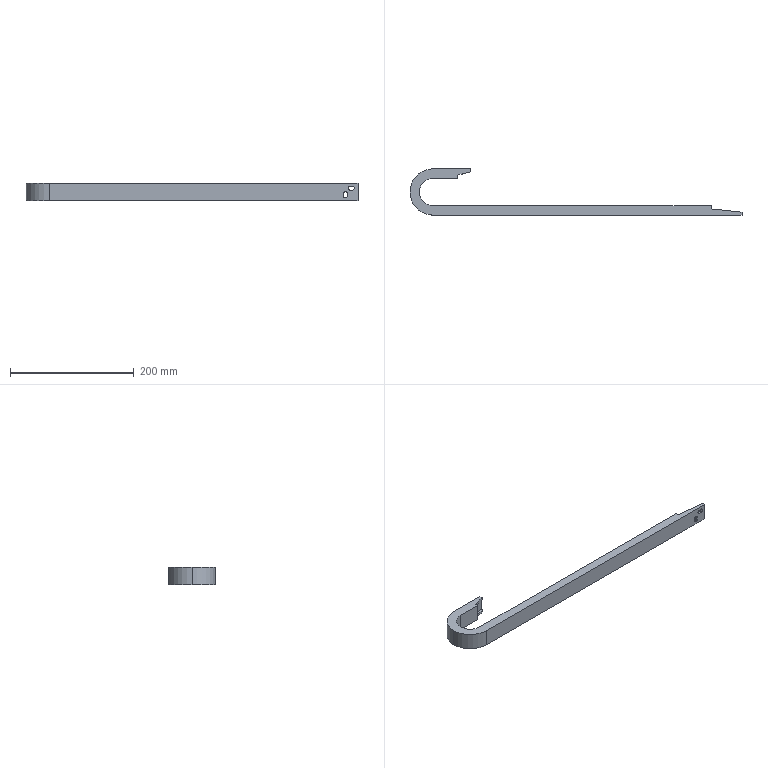Part | SolidWorks | features BaseBody 1 | 1 solid | 46 faces | box 537.6 x 75.2 x 28 mm | volume 139121 mm3 | plane 28 | cylinder 18 | commonest cylinder face diameters 6.5 x10 44.8 x2 50 x2 70 x2 75.2 x2
STEP:
#1=CARTESIAN_POINT('',(-460.45,65.,0.4));
#2=VERTEX_POINT('',#1);
#3=CARTESIAN_POINT('',(-457.2,65.,-2.85));
#4=VERTEX_POINT('',#3);
#5=CARTESIAN_POINT('',(-460.45,65.,-2.85));
#6=DIRECTION('',(0.,1.,0.));
#7=DIRECTION('',(0.,0.,-1.));
#8=AXIS2_PLACEMENT_3D('',#5,#6,#7);
#9=CIRCLE('',#8,3.25);
#10=EDGE_CURVE('',#2,#4,#9,.T.);
#11=ORIENTED_EDGE('',*,*,#10,.F.);
#12=CARTESIAN_POINT('',(-460.45,67.6,0.4));
#13=VERTEX_POINT('',#12);
#14=CARTESIAN_POINT('',(-460.45,-7.601,0.4));
#15=DIRECTION('',(0.,1.,0.));
#16=VECTOR('',#15,1000.);
#17=LINE('',#14,#16);
#18=EDGE_CURVE('',#2,#13,#17,.T.);
#19=ORIENTED_EDGE('',*,*,#18,.T.);
#20=CARTESIAN_POINT('',(-457.2,67.6,-2.85));
#21=VERTEX_POINT('',#20);
#22=CARTESIAN_POINT('',(-460.45,67.6,-2.85));
#23=DIRECTION('',(0.,1.,0.));
#24=DIRECTION('',(0.,0.,1.));
#25=AXIS2_PLACEMENT_3D('',#22,#23,#24);
#26=CIRCLE('',#25,3.25);
#27=EDGE_CURVE('',#13,#21,#26,.T.);
#28=ORIENTED_EDGE('',*,*,#27,.T.);
#29=CARTESIAN_POINT('',(-457.2,-7.601,-2.85));
#30=DIRECTION('',(0.,1.,0.));
#31=VECTOR('',#30,1000.);
#32=LINE('',#29,#31);
#33=EDGE_CURVE('',#4,#21,#32,.T.);
#34=ORIENTED_EDGE('',*,*,#33,.F.);
#35=EDGE_LOOP('',(#11,#19,#28,#34));
#36=FACE_OUTER_BOUND('',#35,.T.);
#37=CARTESIAN_POINT('',(-460.45,-7.601,-2.85));
#38=DIRECTION('',(0.,1.,0.));
#39=DIRECTION('',(0.,0.,1.));
#40=AXIS2_PLACEMENT_3D('',#37,#38,#39);
#41=CYLINDRICAL_SURFACE('',#40,3.25);
#42=ADVANCED_FACE('',(#36),#41,.F.);
#43=CARTESIAN_POINT('',(-20.45,-7.6,0.4));
#44=VERTEX_POINT('',#43);
#45=CARTESIAN_POINT('',(-17.2,-7.6,-2.85));
#46=VERTEX_POINT('',#45);
#47=CARTESIAN_POINT('',(-20.45,-7.6,-2.85));
#48=DIRECTION('',(0.,1.,0.));
#49=DIRECTION('',(0.,0.,1.));
#50=AXIS2_PLACEMENT_3D('',#47,#48,#49);
#51=CIRCLE('',#50,3.25);
#52=EDGE_CURVE('',#44,#46,#51,.T.);
#53=ORIENTED_EDGE('',*,*,#52,.F.);
#54=CARTESIAN_POINT('',(-20.45,-5.,0.4));
#55=VERTEX_POINT('',#54);
#56=CARTESIAN_POINT('',(-20.45,-7.6,0.4));
#57=DIRECTION('',(0.,1.,0.));
#58=VECTOR('',#57,1000.);
#59=LINE('',#56,#58);
#60=EDGE_CURVE('',#44,#55,#59,.T.);
#61=ORIENTED_EDGE('',*,*,#60,.T.);
#62=CARTESIAN_POINT('',(-17.2,-5.,-2.85));
#63=VERTEX_POINT('',#62);
#64=CARTESIAN_POINT('',(-20.45,-5.,-2.85));
#65=DIRECTION('',(0.,1.,0.));
#66=DIRECTION('',(0.,0.,1.));
#67=AXIS2_PLACEMENT_3D('',#64,#65,#66);
#68=CIRCLE('',#67,3.25);
#69=EDGE_CURVE('',#55,#63,#68,.T.);
#70=ORIENTED_EDGE('',*,*,#69,.T.);
#71=CARTESIAN_POINT('',(-17.2,-7.6,-2.85));
#72=DIRECTION('',(0.,1.,0.));
#73=VECTOR('',#72,1000.);
#74=LINE('',#71,#73);
#75=EDGE_CURVE('',#46,#63,#74,.T.);
#76=ORIENTED_EDGE('',*,*,#75,.F.);
#77=EDGE_LOOP('',(#53,#61,#70,#76));
#78=FACE_OUTER_BOUND('',#77,.T.);
#79=CARTESIAN_POINT('',(-20.45,-7.6,-2.85));
#80=DIRECTION('',(0.,1.,0.));
#81=DIRECTION('',(0.,0.,1.));
#82=AXIS2_PLACEMENT_3D('',#79,#80,#81);
#83=CYLINDRICAL_SURFACE('',#82,3.25);
#84=ADVANCED_FACE('',(#78),#83,.F.);
#85=CARTESIAN_POINT('',(-500.,-7.6,14.));
#86=VERTEX_POINT('',#85);
#87=CARTESIAN_POINT('',(-537.6,30.,14.));
#88=VERTEX_POINT('',#87);
#89=CARTESIAN_POINT('',(-500.,30.,14.));
#90=DIRECTION('',(0.,0.,-1.));
#91=DIRECTION('',(-1.,0.,0.));
#92=AXIS2_PLACEMENT_3D('',#89,#90,#91);
#93=CIRCLE('',#92,37.6);
#94=EDGE_CURVE('',#86,#88,#93,.T.);
#95=ORIENTED_EDGE('',*,*,#94,.T.);
#96=CARTESIAN_POINT('',(-537.6,30.,-14.));
#97=VERTEX_POINT('',#96);
#98=CARTESIAN_POINT('',(-537.6,30.,0.));
#99=DIRECTION('',(0.,0.,-1.));
#100=VECTOR('',#99,1000.);
#101=LINE('',#98,#100);
#102=EDGE_CURVE('',#88,#97,#101,.T.);
#103=ORIENTED_EDGE('',*,*,#102,.T.);
#104=CARTESIAN_POINT('',(-500.,-7.6,-14.));
#105=VERTEX_POINT('',#104);
#106=CARTESIAN_POINT('',(-500.,30.,-14.));
#107=DIRECTION('',(0.,0.,-1.));
#108=DIRECTION('',(-1.,0.,0.));
#109=AXIS2_PLACEMENT_3D('',#106,#107,#108);
#110=CIRCLE('',#109,37.6);
#111=EDGE_CURVE('',#105,#97,#110,.T.);
#112=ORIENTED_EDGE('',*,*,#111,.F.);
#113=CARTESIAN_POINT('',(-500.,-7.6,-14.));
#114=DIRECTION('',(0.,0.,-1.));
#115=VECTOR('',#114,1000.);
#116=LINE('',#113,#115);
#117=EDGE_CURVE('',#86,#105,#116,.T.);
#118=ORIENTED_EDGE('',*,*,#117,.F.);
#119=EDGE_LOOP('',(#95,#103,#112,#118));
#120=FACE_OUTER_BOUND('',#119,.T.);
#121=CARTESIAN_POINT('',(-500.,30.,0.));
#122=DIRECTION('',(0.,0.,-1.));
#123=DIRECTION('',(-1.,0.,0.));
#124=AXIS2_PLACEMENT_3D('',#121,#122,#123);
#125=CYLINDRICAL_SURFACE('',#124,37.6);
#126=ADVANCED_FACE('',(#120),#125,.T.);
#127=CARTESIAN_POINT('',(-522.4,30.,14.));
#128=VERTEX_POINT('',#127);
#129=CARTESIAN_POINT('',(-500.,52.4,14.));
#130=VERTEX_POINT('',#129);
#131=CARTESIAN_POINT('',(-500.,30.,14.));
#132=DIRECTION('',(0.,0.,-1.));
#133=DIRECTION('',(-1.,0.,0.));
#134=AXIS2_PLACEMENT_3D('',#131,#132,#133);
#135=CIRCLE('',#134,22.4);
#136=EDGE_CURVE('',#128,#130,#135,.T.);
#137=ORIENTED_EDGE('',*,*,#136,.F.);
#138=CARTESIAN_POINT('',(-522.4,30.,-14.));
#139=VERTEX_POINT('',#138);
#140=CARTESIAN_POINT('',(-522.4,30.,0.));
#141=DIRECTION('',(0.,0.,-1.));
#142=VECTOR('',#141,1000.);
#143=LINE('',#140,#142);
#144=EDGE_CURVE('',#128,#139,#143,.T.);
#145=ORIENTED_EDGE('',*,*,#144,.T.);
#146=CARTESIAN_POINT('',(-500.,52.4,-14.));
#147=VERTEX_POINT('',#146);
#148=CARTESIAN_POINT('',(-500.,30.,-14.));
#149=DIRECTION('',(0.,0.,-1.));
#150=DIRECTION('',(-1.,0.,0.));
#151=AXIS2_PLACEMENT_3D('',#148,#149,#150);
#152=CIRCLE('',#151,22.4);
#153=EDGE_CURVE('',#139,#147,#152,.T.);
#154=ORIENTED_EDGE('',*,*,#153,.T.);
#155=CARTESIAN_POINT('',(-500.,52.4,-14.));
#156=DIRECTION('',(0.,0.,1.));
#157=VECTOR('',#156,1000.);
#158=LINE('',#155,#157);
#159=EDGE_CURVE('',#147,#130,#158,.T.);
#160=ORIENTED_EDGE('',*,*,#159,.T.);
#161=EDGE_LOOP('',(#137,#145,#154,#160));
#162=FACE_OUTER_BOUND('',#161,.T.);
#163=CARTESIAN_POINT('',(-500.,30.,0.));
#164=DIRECTION('',(0.,0.,-1.));
#165=DIRECTION('',(-1.,0.,0.));
#166=AXIS2_PLACEMENT_3D('',#163,#164,#165);
#167=CYLINDRICAL_SURFACE('',#166,22.4);
#168=ADVANCED_FACE('',(#162),#167,.F.);
#169=CARTESIAN_POINT('',(-500.,5.,10.));
#170=VERTEX_POINT('',#169);
#171=CARTESIAN_POINT('',(-525.,30.,10.));
#172=VERTEX_POINT('',#171);
#173=CARTESIAN_POINT('',(-500.,30.,10.));
#174=DIRECTION('',(0.,0.,-1.));
#175=DIRECTION('',(-1.,0.,0.));
#176=AXIS2_PLACEMENT_3D('',#173,#174,#175);
#177=CIRCLE('',#176,25.);
#178=EDGE_CURVE('',#170,#172,#177,.T.);
#179=ORIENTED_EDGE('',*,*,#178,.T.);
#180=CARTESIAN_POINT('',(-525.,30.,-10.));
#181=VERTEX_POINT('',#180);
#182=CARTESIAN_POINT('',(-525.,30.,0.));
#183=DIRECTION('',(0.,0.,-1.));
#184=VECTOR('',#183,1000.);
#185=LINE('',#182,#184);
#186=EDGE_CURVE('',#172,#181,#185,.T.);
#187=ORIENTED_EDGE('',*,*,#186,.T.);
#188=CARTESIAN_POINT('',(-500.,5.,-10.));
#189=VERTEX_POINT('',#188);
#190=CARTESIAN_POINT('',(-500.,30.,-10.));
#191=DIRECTION('',(0.,0.,-1.));
#192=DIRECTION('',(-1.,0.,0.));
#193=AXIS2_PLACEMENT_3D('',#190,#191,#192);
#194=CIRCLE('',#193,25.);
#195=EDGE_CURVE('',#189,#181,#194,.T.);
#196=ORIENTED_EDGE('',*,*,#195,.F.);
#197=CARTESIAN_POINT('',(-500.,5.,-10.));
#198=DIRECTION('',(0.,0.,1.));
#199=VECTOR('',#198,1000.);
#200=LINE('',#197,#199);
#201=EDGE_CURVE('',#189,#170,#200,.T.);
#202=ORIENTED_EDGE('',*,*,#201,.T.);
#203=EDGE_LOOP('',(#179,#187,#196,#202));
#204=FACE_OUTER_BOUND('',#203,.T.);
#205=CARTESIAN_POINT('',(-500.,30.,0.));
#206=DIRECTION('',(0.,0.,-1.));
#207=DIRECTION('',(-1.,0.,0.));
#208=AXIS2_PLACEMENT_3D('',#205,#206,#207);
#209=CYLINDRICAL_SURFACE('',#208,25.);
#210=ADVANCED_FACE('',(#204),#209,.T.);
#211=CARTESIAN_POINT('',(-535.,30.,10.));
#212=VERTEX_POINT('',#211);
#213=CARTESIAN_POINT('',(-500.,65.,10.));
#214=VERTEX_POINT('',#213);
#215=CARTESIAN_POINT('',(-500.,30.,10.));
#216=DIRECTION('',(0.,0.,-1.));
#217=DIRECTION('',(-1.,0.,0.));
#218=AXIS2_PLACEMENT_3D('',#215,#216,#217);
#219=CIRCLE('',#218,35.);
#220=EDGE_CURVE('',#212,#214,#219,.T.);
#221=ORIENTED_EDGE('',*,*,#220,.F.);
#222=CARTESIAN_POINT('',(-535.,30.,-10.));
#223=VERTEX_POINT('',#222);
#224=CARTESIAN_POINT('',(-535.,30.,0.));
#225=DIRECTION('',(0.,0.,-1.));
#226=VECTOR('',#225,1000.);
#227=LINE('',#224,#226);
#228=EDGE_CURVE('',#212,#223,#227,.T.);
#229=ORIENTED_EDGE('',*,*,#228,.T.);
#230=CARTESIAN_POINT('',(-500.,65.,-10.));
#231=VERTEX_POINT('',#230);
#232=CARTESIAN_POINT('',(-500.,30.,-10.));
#233=DIRECTION('',(0.,0.,-1.));
#234=DIRECTION('',(-1.,0.,0.));
#235=AXIS2_PLACEMENT_3D('',#232,#233,#234);
#236=CIRCLE('',#235,35.);
#237=EDGE_CURVE('',#223,#231,#236,.T.);
#238=ORIENTED_EDGE('',*,*,#237,.T.);
#239=CARTESIAN_POINT('',(-500.,65.,-10.));
#240=DIRECTION('',(0.,0.,-1.));
#241=VECTOR('',#240,1000.);
#242=LINE('',#239,#241);
#243=EDGE_CURVE('',#214,#231,#242,.T.);
#244=ORIENTED_EDGE('',*,*,#243,.F.);
#245=EDGE_LOOP('',(#221,#229,#238,#244));
#246=FACE_OUTER_BOUND('',#245,.T.);
#247=CARTESIAN_POINT('',(-500.,30.,0.));
#248=DIRECTION('',(0.,0.,-1.));
#249=DIRECTION('',(-1.,0.,0.));
#250=AXIS2_PLACEMENT_3D('',#247,#248,#249);
#251=CYLINDRICAL_SURFACE('',#250,35.);
#252=ADVANCED_FACE('',(#246),#251,.F.);
#253=CARTESIAN_POINT('',(-452.75,65.,3.1));
#254=VERTEX_POINT('',#253);
#255=CARTESIAN_POINT('',(-452.75,65.,9.6));
#256=VERTEX_POINT('',#255);
#257=CARTESIAN_POINT('',(-452.75,65.,6.35));
#258=DIRECTION('',(0.,1.,0.));
#259=DIRECTION('',(0.,0.,-1.));
#260=AXIS2_PLACEMENT_3D('',#257,#258,#259);
#261=CIRCLE('',#260,3.25);
#262=EDGE_CURVE('',#254,#256,#261,.T.);
#263=ORIENTED_EDGE('',*,*,#262,.T.);
#264=CARTESIAN_POINT('',(-449.25,65.,9.6));
#265=VERTEX_POINT('',#264);
#266=CARTESIAN_POINT('',(-452.75,65.,9.6));
#267=DIRECTION('',(1.,0.,0.));
#268=VECTOR('',#267,1000.);
#269=LINE('',#266,#268);
#270=EDGE_CURVE('',#256,#265,#269,.T.);
#271=ORIENTED_EDGE('',*,*,#270,.T.);
#272=CARTESIAN_POINT('',(-449.25,65.,3.1));
#273=VERTEX_POINT('',#272);
#274=CARTESIAN_POINT('',(-449.25,65.,6.35));
#275=DIRECTION('',(0.,1.,0.));
#276=DIRECTION('',(0.,0.,-1.));
#277=AXIS2_PLACEMENT_3D('',#274,#275,#276);
#278=CIRCLE('',#277,3.25);
#279=EDGE_CURVE('',#265,#273,#278,.T.);
#280=ORIENTED_EDGE('',*,*,#279,.T.);
#281=CARTESIAN_POINT('',(-452.75,65.,3.1));
#282=DIRECTION('',(-1.,0.,0.));
#283=VECTOR('',#282,1000.);
#284=LINE('',#281,#283);
#285=EDGE_CURVE('',#273,#254,#284,.T.);
#286=ORIENTED_EDGE('',*,*,#285,.T.);
#287=EDGE_LOOP('',(#263,#271,#280,#286));
#288=FACE_BOUND('',#287,.T.);
#289=CARTESIAN_POINT('',(-457.2,65.,-6.35));
#290=VERTEX_POINT('',#289);
#291=CARTESIAN_POINT('',(-463.7,65.,-6.35));
#292=VERTEX_POINT('',#291);
#293=CARTESIAN_POINT('',(-460.45,65.,-6.35));
#294=DIRECTION('',(0.,1.,0.));
#295=DIRECTION('',(0.,0.,-1.));
#296=AXIS2_PLACEMENT_3D('',#293,#294,#295);
#297=CIRCLE('',#296,3.25);
#298=EDGE_CURVE('',#290,#292,#297,.T.);
#299=ORIENTED_EDGE('',*,*,#298,.T.);
#300=CARTESIAN_POINT('',(-463.7,65.,-2.85));
#301=VERTEX_POINT('',#300);
#302=CARTESIAN_POINT('',(-463.7,65.,-6.35));
#303=DIRECTION('',(0.,0.,1.));
#304=VECTOR('',#303,1000.);
#305=LINE('',#302,#304);
#306=EDGE_CURVE('',#292,#301,#305,.T.);
#307=ORIENTED_EDGE('',*,*,#306,.T.);
#308=CARTESIAN_POINT('',(-460.45,65.,-2.85));
#309=DIRECTION('',(0.,1.,0.));
#310=DIRECTION('',(0.,0.,-1.));
#311=AXIS2_PLACEMENT_3D('',#308,#309,#310);
#312=CIRCLE('',#311,3.25);
#313=EDGE_CURVE('',#301,#2,#312,.T.);
#314=ORIENTED_EDGE('',*,*,#313,.T.);
#315=ORIENTED_EDGE('',*,*,#10,.T.);
#316=CARTESIAN_POINT('',(-457.2,65.,-6.35));
#317=DIRECTION('',(0.,0.,-1.));
#318=VECTOR('',#317,1000.);
#319=LINE('',#316,#318);
#320=EDGE_CURVE('',#4,#290,#319,.T.);
#321=ORIENTED_EDGE('',*,*,#320,.T.);
#322=EDGE_LOOP('',(#299,#307,#314,#315,#321));
#323=FACE_BOUND('',#322,.T.);
#324=ORIENTED_EDGE('',*,*,#243,.T.);
#325=CARTESIAN_POINT('',(-440.,65.,-10.));
#326=VERTEX_POINT('',#325);
#327=CARTESIAN_POINT('',(-500.,65.,-10.));
#328=DIRECTION('',(1.,0.,0.));
#329=VECTOR('',#328,1000.);
#330=LINE('',#327,#329);
#331=EDGE_CURVE('',#231,#326,#330,.T.);
#332=ORIENTED_EDGE('',*,*,#331,.T.);
#333=CARTESIAN_POINT('',(-440.,65.,10.));
#334=VERTEX_POINT('',#333);
#335=CARTESIAN_POINT('',(-440.,65.,-10.));
#336=DIRECTION('',(0.,0.,-1.));
#337=VECTOR('',#336,1000.);
#338=LINE('',#335,#337);
#339=EDGE_CURVE('',#334,#326,#338,.T.);
#340=ORIENTED_EDGE('',*,*,#339,.F.);
#341=CARTESIAN_POINT('',(-500.,65.,10.));
#342=DIRECTION('',(1.,0.,0.));
#343=VECTOR('',#342,1000.);
#344=LINE('',#341,#343);
#345=EDGE_CURVE('',#214,#334,#344,.T.);
#346=ORIENTED_EDGE('',*,*,#345,.F.);
#347=EDGE_LOOP('',(#324,#332,#340,#346));
#348=FACE_OUTER_BOUND('',#347,.T.);
#349=CARTESIAN_POINT('',(-500.,65.,-10.));
#350=DIRECTION('',(0.,-1.,0.));
#351=DIRECTION('',(0.,0.,-1.));
#352=AXIS2_PLACEMENT_3D('',#349,#350,#351);
#353=PLANE('',#352);
#354=ADVANCED_FACE('',(#288,#323,#348),#353,.T.);
#355=CARTESIAN_POINT('',(-460.,55.,-10.));
#356=VERTEX_POINT('',#355);
#357=CARTESIAN_POINT('',(-460.,55.,10.));
#358=VERTEX_POINT('',#357);
#359=CARTESIAN_POINT('',(-460.,55.,-10.));
#360=DIRECTION('',(0.,0.,1.));
#361=VECTOR('',#360,1000.);
#362=LINE('',#359,#361);
#363=EDGE_CURVE('',#356,#358,#362,.T.);
#364=ORIENTED_EDGE('',*,*,#363,.F.);
#365=CARTESIAN_POINT('',(-500.,55.,-10.));
#366=VERTEX_POINT('',#365);
#367=CARTESIAN_POINT('',(-500.,55.,-10.));
#368=DIRECTION('',(1.,0.,0.));
#369=VECTOR('',#368,1000.);
#370=LINE('',#367,#369);
#371=EDGE_CURVE('',#366,#356,#370,.T.);
#372=ORIENTED_EDGE('',*,*,#371,.F.);
#373=CARTESIAN_POINT('',(-500.,55.,10.));
#374=VERTEX_POINT('',#373);
#375=CARTESIAN_POINT('',(-500.,55.,-10.));
#376=DIRECTION('',(0.,0.,1.));
#377=VECTOR('',#376,1000.);
#378=LINE('',#375,#377);
#379=EDGE_CURVE('',#366,#374,#378,.T.);
#380=ORIENTED_EDGE('',*,*,#379,.T.);
#381=CARTESIAN_POINT('',(-500.,55.,10.));
#382=DIRECTION('',(1.,0.,0.));
#383=VECTOR('',#382,1000.);
#384=LINE('',#381,#383);
#385=EDGE_CURVE('',#374,#358,#384,.T.);
#386=ORIENTED_EDGE('',*,*,#385,.T.);
#387=EDGE_LOOP('',(#364,#372,#380,#386));
#388=FACE_OUTER_BOUND('',#387,.T.);
#389=CARTESIAN_POINT('',(-500.,55.,-10.));
#390=DIRECTION('',(0.,1.,0.));
#391=DIRECTION('',(0.,0.,1.));
#392=AXIS2_PLACEMENT_3D('',#389,#390,#391);
#393=PLANE('',#392);
#394=ADVANCED_FACE('',(#388),#393,.T.);
#395=CARTESIAN_POINT('',(-460.,52.4,-14.));
#396=VERTEX_POINT('',#395);
#397=CARTESIAN_POINT('',(-500.,52.4,-14.));
#398=DIRECTION('',(1.,0.,0.));
#399=VECTOR('',#398,1000.);
#400=LINE('',#397,#399);
#401=EDGE_CURVE('',#147,#396,#400,.T.);
#402=ORIENTED_EDGE('',*,*,#401,.T.);
#403=CARTESIAN_POINT('',(-460.,52.4,14.));
#404=VERTEX_POINT('',#403);
#405=CARTESIAN_POINT('',(-460.,52.4,-14.));
#406=DIRECTION('',(0.,0.,1.));
#407=VECTOR('',#406,1000.);
#408=LINE('',#405,#407);
#409=EDGE_CURVE('',#396,#404,#408,.T.);
#410=ORIENTED_EDGE('',*,*,#409,.T.);
#411=CARTESIAN_POINT('',(-500.,52.4,14.));
#412=DIRECTION('',(1.,0.,0.));
#413=VECTOR('',#412,1000.);
#414=LINE('',#411,#413);
#415=EDGE_CURVE('',#130,#404,#414,.T.);
#416=ORIENTED_EDGE('',*,*,#415,.F.);
#417=ORIENTED_EDGE('',*,*,#159,.F.);
#418=EDGE_LOOP('',(#402,#410,#416,#417));
#419=FACE_OUTER_BOUND('',#418,.T.);
#420=CARTESIAN_POINT('',(-500.,52.4,-14.));
#421=DIRECTION('',(0.,1.,0.));
#422=DIRECTION('',(0.,0.,1.));
#423=AXIS2_PLACEMENT_3D('',#420,#421,#422);
#424=PLANE('',#423);
#425=ADVANCED_FACE('',(#419),#424,.F.);
#426=CARTESIAN_POINT('',(-452.75,67.6,9.6));
#427=VERTEX_POINT('',#426);
#428=CARTESIAN_POINT('',(-449.25,67.6,9.6));
#429=VERTEX_POINT('',#428);
#430=CARTESIAN_POINT('',(-452.75,67.6,9.6));
#431=DIRECTION('',(1.,0.,0.));
#432=VECTOR('',#431,1000.);
#433=LINE('',#430,#432);
#434=EDGE_CURVE('',#427,#429,#433,.T.);
#435=ORIENTED_EDGE('',*,*,#434,.F.);
#436=CARTESIAN_POINT('',(-452.75,67.6,3.1));
#437=VERTEX_POINT('',#436);
#438=CARTESIAN_POINT('',(-452.75,67.6,6.35));
#439=DIRECTION('',(0.,1.,0.));
#440=DIRECTION('',(0.,0.,1.));
#441=AXIS2_PLACEMENT_3D('',#438,#439,#440);
#442=CIRCLE('',#441,3.25);
#443=EDGE_CURVE('',#437,#427,#442,.T.);
#444=ORIENTED_EDGE('',*,*,#443,.F.);
#445=CARTESIAN_POINT('',(-449.25,67.6,3.1));
#446=VERTEX_POINT('',#445);
#447=CARTESIAN_POINT('',(-452.75,67.6,3.1));
#448=DIRECTION('',(-1.,0.,0.));
#449=VECTOR('',#448,1000.);
#450=LINE('',#447,#449);
#451=EDGE_CURVE('',#446,#437,#450,.T.);
#452=ORIENTED_EDGE('',*,*,#451,.F.);
#453=CARTESIAN_POINT('',(-449.25,67.6,6.35));
#454=DIRECTION('',(0.,1.,0.));
#455=DIRECTION('',(0.,0.,1.));
#456=AXIS2_PLACEMENT_3D('',#453,#454,#455);
#457=CIRCLE('',#456,3.25);
#458=EDGE_CURVE('',#429,#446,#457,.T.);
#459=ORIENTED_EDGE('',*,*,#458,.F.);
#460=EDGE_LOOP('',(#435,#444,#452,#459));
#461=FACE_BOUND('',#460,.T.);
#462=CARTESIAN_POINT('',(-463.7,67.6,-6.35));
#463=VERTEX_POINT('',#462);
#464=CARTESIAN_POINT('',(-463.7,67.6,-2.85));
#465=VERTEX_POINT('',#464);
#466=CARTESIAN_POINT('',(-463.7,67.6,-6.35));
#467=DIRECTION('',(0.,0.,1.));
#468=VECTOR('',#467,1000.);
#469=LINE('',#466,#468);
#470=EDGE_CURVE('',#463,#465,#469,.T.);
#471=ORIENTED_EDGE('',*,*,#470,.F.);
#472=CARTESIAN_POINT('',(-457.2,67.6,-6.35));
#473=VERTEX_POINT('',#472);
#474=CARTESIAN_POINT('',(-460.45,67.6,-6.35));
#475=DIRECTION('',(0.,1.,0.));
#476=DIRECTION('',(0.,0.,1.));
#477=AXIS2_PLACEMENT_3D('',#474,#475,#476);
#478=CIRCLE('',#477,3.25);
#479=EDGE_CURVE('',#473,#463,#478,.T.);
#480=ORIENTED_EDGE('',*,*,#479,.F.);
#481=CARTESIAN_POINT('',(-457.2,67.6,-6.35));
#482=DIRECTION('',(0.,0.,-1.));
#483=VECTOR('',#482,1000.);
#484=LINE('',#481,#483);
#485=EDGE_CURVE('',#21,#473,#484,.T.);
#486=ORIENTED_EDGE('',*,*,#485,.F.);
#487=ORIENTED_EDGE('',*,*,#27,.F.);
#488=CARTESIAN_POINT('',(-460.45,67.6,-2.85));
#489=DIRECTION('',(0.,1.,0.));
#490=DIRECTION('',(0.,0.,1.));
#491=AXIS2_PLACEMENT_3D('',#488,#489,#490);
#492=CIRCLE('',#491,3.25);
#493=EDGE_CURVE('',#465,#13,#492,.T.);
#494=ORIENTED_EDGE('',*,*,#493,.F.);
#495=EDGE_LOOP('',(#471,#480,#486,#487,#494));
#496=FACE_BOUND('',#495,.T.);
#497=CARTESIAN_POINT('',(-500.,67.6,14.));
#498=VERTEX_POINT('',#497);
#499=CARTESIAN_POINT('',(-500.,67.6,-14.));
#500=VERTEX_POINT('',#499);
#501=CARTESIAN_POINT('',(-500.,67.6,-14.));
#502=DIRECTION('',(0.,0.,-1.));
#503=VECTOR('',#502,1000.);
#504=LINE('',#501,#503);
#505=EDGE_CURVE('',#498,#500,#504,.T.);
#506=ORIENTED_EDGE('',*,*,#505,.F.);
#507=CARTESIAN_POINT('',(-440.,67.6,14.));
#508=VERTEX_POINT('',#507);
#509=CARTESIAN_POINT('',(-500.,67.6,14.));
#510=DIRECTION('',(1.,0.,0.));
#511=VECTOR('',#510,1000.);
#512=LINE('',#509,#511);
#513=EDGE_CURVE('',#498,#508,#512,.T.);
#514=ORIENTED_EDGE('',*,*,#513,.T.);
#515=CARTESIAN_POINT('',(-440.,67.6,-14.));
#516=VERTEX_POINT('',#515);
#517=CARTESIAN_POINT('',(-440.,67.6,-14.));
#518=DIRECTION('',(0.,0.,-1.));
#519=VECTOR('',#518,1000.);
#520=LINE('',#517,#519);
#521=EDGE_CURVE('',#508,#516,#520,.T.);
#522=ORIENTED_EDGE('',*,*,#521,.T.);
#523=CARTESIAN_POINT('',(-500.,67.6,-14.));
#524=DIRECTION('',(1.,0.,0.));
#525=VECTOR('',#524,1000.);
#526=LINE('',#523,#525);
#527=EDGE_CURVE('',#500,#516,#526,.T.);
#528=ORIENTED_EDGE('',*,*,#527,.F.);
#529=EDGE_LOOP('',(#506,#514,#522,#528));
#530=FACE_OUTER_BOUND('',#529,.T.);
#531=CARTESIAN_POINT('',(-500.,67.6,-14.));
#532=DIRECTION('',(0.,-1.,0.));
#533=DIRECTION('',(0.,0.,-1.));
#534=AXIS2_PLACEMENT_3D('',#531,#532,#533);
#535=PLANE('',#534);
#536=ADVANCED_FACE('',(#461,#496,#530),#535,.F.);
#537=ORIENTED_EDGE('',*,*,#228,.F.);
#538=CARTESIAN_POINT('',(-500.,-5.,10.));
#539=VERTEX_POINT('',#538);
#540=CARTESIAN_POINT('',(-500.,30.,10.));
#541=DIRECTION('',(0.,0.,-1.));
#542=DIRECTION('',(-1.,0.,0.));
#543=AXIS2_PLACEMENT_3D('',#540,#541,#542);
#544=CIRCLE('',#543,35.);
#545=EDGE_CURVE('',#539,#212,#544,.T.);
#546=ORIENTED_EDGE('',*,*,#545,.F.);
#547=CARTESIAN_POINT('',(-500.,-5.,-10.));
#548=VERTEX_POINT('',#547);
#549=CARTESIAN_POINT('',(-500.,-5.,-10.));
#550=DIRECTION('',(0.,0.,-1.));
#551=VECTOR('',#550,1000.);
#552=LINE('',#549,#551);
#553=EDGE_CURVE('',#539,#548,#552,.T.);
#554=ORIENTED_EDGE('',*,*,#553,.T.);
#555=CARTESIAN_POINT('',(-500.,30.,-10.));
#556=DIRECTION('',(0.,0.,-1.));
#557=DIRECTION('',(-1.,0.,0.));
#558=AXIS2_PLACEMENT_3D('',#555,#556,#557);
#559=CIRCLE('',#558,35.);
#560=EDGE_CURVE('',#548,#223,#559,.T.);
#561=ORIENTED_EDGE('',*,*,#560,.T.);
#562=EDGE_LOOP('',(#537,#546,#554,#561));
#563=FACE_OUTER_BOUND('',#562,.T.);
#564=CARTESIAN_POINT('',(-500.,30.,0.));
#565=DIRECTION('',(0.,0.,-1.));
#566=DIRECTION('',(-1.,0.,0.));
#567=AXIS2_PLACEMENT_3D('',#564,#565,#566);
#568=CYLINDRICAL_SURFACE('',#567,35.);
#569=ADVANCED_FACE('',(#563),#568,.F.);
#570=ORIENTED_EDGE('',*,*,#186,.F.);
#571=CARTESIAN_POINT('',(-500.,30.,10.));
#572=DIRECTION('',(0.,0.,-1.));
#573=DIRECTION('',(-1.,0.,0.));
#574=AXIS2_PLACEMENT_3D('',#571,#572,#573);
#575=CIRCLE('',#574,25.);
#576=EDGE_CURVE('',#172,#374,#575,.T.);
#577=ORIENTED_EDGE('',*,*,#576,.T.);
#578=ORIENTED_EDGE('',*,*,#379,.F.);
#579=CARTESIAN_POINT('',(-500.,30.,-10.));
#580=DIRECTION('',(0.,0.,-1.));
#581=DIRECTION('',(-1.,0.,0.));
#582=AXIS2_PLACEMENT_3D('',#579,#580,#581);
#583=CIRCLE('',#582,25.);
#584=EDGE_CURVE('',#181,#366,#583,.T.);
#585=ORIENTED_EDGE('',*,*,#584,.F.);
#586=EDGE_LOOP('',(#570,#577,#578,#585));
#587=FACE_OUTER_BOUND('',#586,.T.);
#588=CARTESIAN_POINT('',(-500.,30.,0.));
#589=DIRECTION('',(0.,0.,-1.));
#590=DIRECTION('',(-1.,0.,0.));
#591=AXIS2_PLACEMENT_3D('',#588,#589,#590);
#592=CYLINDRICAL_SURFACE('',#591,25.);
#593=ADVANCED_FACE('',(#587),#592,.T.);
#594=ORIENTED_EDGE('',*,*,#144,.F.);
#595=CARTESIAN_POINT('',(-500.,7.6,14.));
#596=VERTEX_POINT('',#595);
#597=CARTESIAN_POINT('',(-500.,30.,14.));
#598=DIRECTION('',(0.,0.,-1.));
#599=DIRECTION('',(-1.,0.,0.));
#600=AXIS2_PLACEMENT_3D('',#597,#598,#599);
#601=CIRCLE('',#600,22.4);
#602=EDGE_CURVE('',#596,#128,#601,.T.);
#603=ORIENTED_EDGE('',*,*,#602,.F.);
#604=CARTESIAN_POINT('',(-500.,7.6,-14.));
#605=VERTEX_POINT('',#604);
#606=CARTESIAN_POINT('',(-500.,7.6,-14.));
#607=DIRECTION('',(0.,0.,1.));
#608=VECTOR('',#607,1000.);
#609=LINE('',#606,#608);
#610=EDGE_CURVE('',#605,#596,#609,.T.);
#611=ORIENTED_EDGE('',*,*,#610,.F.);
#612=CARTESIAN_POINT('',(-500.,30.,-14.));
#613=DIRECTION('',(0.,0.,-1.));
#614=DIRECTION('',(-1.,0.,0.));
#615=AXIS2_PLACEMENT_3D('',#612,#613,#614);
#616=CIRCLE('',#615,22.4);
#617=EDGE_CURVE('',#605,#139,#616,.T.);
#618=ORIENTED_EDGE('',*,*,#617,.T.);
#619=EDGE_LOOP('',(#594,#603,#611,#618));
#620=FACE_OUTER_BOUND('',#619,.T.);
#621=CARTESIAN_POINT('',(-500.,30.,0.));
#622=DIRECTION('',(0.,0.,-1.));
#623=DIRECTION('',(-1.,0.,0.));
#624=AXIS2_PLACEMENT_3D('',#621,#622,#623);
#625=CYLINDRICAL_SURFACE('',#624,22.4);
#626=ADVANCED_FACE('',(#620),#625,.F.);
#627=ORIENTED_EDGE('',*,*,#102,.F.);
#628=CARTESIAN_POINT('',(-500.,30.,14.));
#629=DIRECTION('',(0.,0.,-1.));
#630=DIRECTION('',(-1.,0.,0.));
#631=AXIS2_PLACEMENT_3D('',#628,#629,#630);
#632=CIRCLE('',#631,37.6);
#633=EDGE_CURVE('',#88,#498,#632,.T.);
#634=ORIENTED_EDGE('',*,*,#633,.T.);
#635=ORIENTED_EDGE('',*,*,#505,.T.);
#636=CARTESIAN_POINT('',(-500.,30.,-14.));
#637=DIRECTION('',(0.,0.,-1.));
#638=DIRECTION('',(-1.,0.,0.));
#639=AXIS2_PLACEMENT_3D('',#636,#637,#638);
#640=CIRCLE('',#639,37.6);
#641=EDGE_CURVE('',#97,#500,#640,.T.);
#642=ORIENTED_EDGE('',*,*,#641,.F.);
#643=EDGE_LOOP('',(#627,#634,#635,#642));
#644=FACE_OUTER_BOUND('',#643,.T.);
#645=CARTESIAN_POINT('',(-500.,30.,0.));
#646=DIRECTION('',(0.,0.,-1.));
#647=DIRECTION('',(-1.,0.,0.));
#648=AXIS2_PLACEMENT_3D('',#645,#646,#647);
#649=CYLINDRICAL_SURFACE('',#648,37.6);
#650=ADVANCED_FACE('',(#644),#649,.T.);
#651=CARTESIAN_POINT('',(-50.,5.,10.));
#652=VERTEX_POINT('',#651);
#653=CARTESIAN_POINT('',(-50.,2.6,10.));
#654=VERTEX_POINT('',#653);
#655=CARTESIAN_POINT('',(-50.,5.,10.));
#656=DIRECTION('',(0.,-1.,0.));
#657=VECTOR('',#656,1000.);
#658=LINE('',#655,#657);
#659=EDGE_CURVE('',#652,#654,#658,.T.);
#660=ORIENTED_EDGE('',*,*,#659,.T.);
#661=CARTESIAN_POINT('',(0.,-2.6,10.));
#662=VERTEX_POINT('',#661);
#663=CARTESIAN_POINT('',(-495.432,48.925,10.));
#664=DIRECTION('',(0.9946,-0.1034,0.));
#665=VECTOR('',#664,1000.);
#666=LINE('',#663,#665);
#667=EDGE_CURVE('',#654,#662,#666,.T.);
#668=ORIENTED_EDGE('',*,*,#667,.T.);
#669=CARTESIAN_POINT('',(0.,-5.,10.));
#670=VERTEX_POINT('',#669);
#671=CARTESIAN_POINT('',(0.,5.,10.));
#672=DIRECTION('',(0.,-1.,0.));
#673=VECTOR('',#672,1000.);
#674=LINE('',#671,#673);
#675=EDGE_CURVE('',#662,#670,#674,.T.);
#676=ORIENTED_EDGE('',*,*,#675,.T.);
#677=CARTESIAN_POINT('',(-500.,-5.,10.));
#678=DIRECTION('',(1.,0.,0.));
#679=VECTOR('',#678,1000.);
#680=LINE('',#677,#679);
#681=EDGE_CURVE('',#539,#670,#680,.T.);
#682=ORIENTED_EDGE('',*,*,#681,.F.);
#683=ORIENTED_EDGE('',*,*,#545,.T.);
#684=ORIENTED_EDGE('',*,*,#220,.T.);
#685=ORIENTED_EDGE('',*,*,#345,.T.);
#686=CARTESIAN_POINT('',(-440.,62.6,10.));
#687=VERTEX_POINT('',#686);
#688=CARTESIAN_POINT('',(-440.,55.,10.));
#689=DIRECTION('',(0.,1.,0.));
#690=VECTOR('',#689,1000.);
#691=LINE('',#688,#690);
#692=EDGE_CURVE('',#687,#334,#691,.T.);
#693=ORIENTED_EDGE('',*,*,#692,.F.);
#694=CARTESIAN_POINT('',(-460.,57.4,10.));
#695=VERTEX_POINT('',#694);
#696=CARTESIAN_POINT('',(-510.229,44.341,10.));
#697=DIRECTION('',(-0.9678,-0.2516,0.));
#698=VECTOR('',#697,1000.);
#699=LINE('',#696,#698);
#700=EDGE_CURVE('',#687,#695,#699,.T.);
#701=ORIENTED_EDGE('',*,*,#700,.T.);
#702=CARTESIAN_POINT('',(-460.,5.,10.));
#703=DIRECTION('',(0.,-1.,0.));
#704=VECTOR('',#703,1000.);
#705=LINE('',#702,#704);
#706=EDGE_CURVE('',#695,#358,#705,.T.);
#707=ORIENTED_EDGE('',*,*,#706,.T.);
#708=ORIENTED_EDGE('',*,*,#385,.F.);
#709=ORIENTED_EDGE('',*,*,#576,.F.);
#710=ORIENTED_EDGE('',*,*,#178,.F.);
#711=CARTESIAN_POINT('',(-500.,5.,10.));
#712=DIRECTION('',(1.,0.,0.));
#713=VECTOR('',#712,1000.);
#714=LINE('',#711,#713);
#715=EDGE_CURVE('',#170,#652,#714,.T.);
#716=ORIENTED_EDGE('',*,*,#715,.T.);
#717=EDGE_LOOP('',(#660,#668,#676,#682,#683,#684,#685,#693,#701,#707,#708,#709,#710,#716));
#718=FACE_OUTER_BOUND('',#717,.T.);
#719=CARTESIAN_POINT('',(-500.,5.,10.));
#720=DIRECTION('',(0.,0.,1.));
#721=DIRECTION('',(0.,-1.,0.));
#722=AXIS2_PLACEMENT_3D('',#719,#720,#721);
#723=PLANE('',#722);
#724=ADVANCED_FACE('',(#718),#723,.F.);
#725=CARTESIAN_POINT('',(-23.7,-5.,-6.35));
#726=VERTEX_POINT('',#725);
#727=CARTESIAN_POINT('',(-23.7,-5.,-2.85));
#728=VERTEX_POINT('',#727);
#729=CARTESIAN_POINT('',(-23.7,-5.,-6.35));
#730=DIRECTION('',(0.,0.,1.));
#731=VECTOR('',#730,1000.);
#732=LINE('',#729,#731);
#733=EDGE_CURVE('',#726,#728,#732,.T.);
#734=ORIENTED_EDGE('',*,*,#733,.F.);
#735=CARTESIAN_POINT('',(-17.2,-5.,-6.35));
#736=VERTEX_POINT('',#735);
#737=CARTESIAN_POINT('',(-20.45,-5.,-6.35));
#738=DIRECTION('',(0.,1.,0.));
#739=DIRECTION('',(0.,0.,1.));
#740=AXIS2_PLACEMENT_3D('',#737,#738,#739);
#741=CIRCLE('',#740,3.25);
#742=EDGE_CURVE('',#736,#726,#741,.T.);
#743=ORIENTED_EDGE('',*,*,#742,.F.);
#744=CARTESIAN_POINT('',(-17.2,-5.,-6.35));
#745=DIRECTION('',(0.,0.,-1.));
#746=VECTOR('',#745,1000.);
#747=LINE('',#744,#746);
#748=EDGE_CURVE('',#63,#736,#747,.T.);
#749=ORIENTED_EDGE('',*,*,#748,.F.);
#750=ORIENTED_EDGE('',*,*,#69,.F.);
#751=CARTESIAN_POINT('',(-20.45,-5.,-2.85));
#752=DIRECTION('',(0.,1.,0.));
#753=DIRECTION('',(0.,0.,1.));
#754=AXIS2_PLACEMENT_3D('',#751,#752,#753);
#755=CIRCLE('',#754,3.25);
#756=EDGE_CURVE('',#728,#55,#755,.T.);
#757=ORIENTED_EDGE('',*,*,#756,.F.);
#758=EDGE_LOOP('',(#734,#743,#749,#750,#757));
#759=FACE_BOUND('',#758,.T.);
#760=CARTESIAN_POINT('',(-12.75,-5.,9.6));
#761=VERTEX_POINT('',#760);
#762=CARTESIAN_POINT('',(-9.25,-5.,9.6));
#763=VERTEX_POINT('',#762);
#764=CARTESIAN_POINT('',(-12.75,-5.,9.6));
#765=DIRECTION('',(1.,0.,0.));
#766=VECTOR('',#765,1000.);
#767=LINE('',#764,#766);
#768=EDGE_CURVE('',#761,#763,#767,.T.);
#769=ORIENTED_EDGE('',*,*,#768,.F.);
#770=CARTESIAN_POINT('',(-12.75,-5.,3.1));
#771=VERTEX_POINT('',#770);
#772=CARTESIAN_POINT('',(-12.75,-5.,6.35));
#773=DIRECTION('',(0.,1.,0.));
#774=DIRECTION('',(0.,0.,1.));
#775=AXIS2_PLACEMENT_3D('',#772,#773,#774);
#776=CIRCLE('',#775,3.25);
#777=EDGE_CURVE('',#771,#761,#776,.T.);
#778=ORIENTED_EDGE('',*,*,#777,.F.);
#779=CARTESIAN_POINT('',(-9.25,-5.,3.1));
#780=VERTEX_POINT('',#779);
#781=CARTESIAN_POINT('',(-12.75,-5.,3.1));
#782=DIRECTION('',(-1.,0.,0.));
#783=VECTOR('',#782,1000.);
#784=LINE('',#781,#783);
#785=EDGE_CURVE('',#780,#771,#784,.T.);
#786=ORIENTED_EDGE('',*,*,#785,.F.);
#787=CARTESIAN_POINT('',(-9.25,-5.,6.35));
#788=DIRECTION('',(0.,1.,0.));
#789=DIRECTION('',(0.,0.,1.));
#790=AXIS2_PLACEMENT_3D('',#787,#788,#789);
#791=CIRCLE('',#790,3.25);
#792=EDGE_CURVE('',#763,#780,#791,.T.);
#793=ORIENTED_EDGE('',*,*,#792,.F.);
#794=EDGE_LOOP('',(#769,#778,#786,#793));
#795=FACE_BOUND('',#794,.T.);
#796=CARTESIAN_POINT('',(0.,-5.,-10.));
#797=VERTEX_POINT('',#796);
#798=CARTESIAN_POINT('',(0.,-5.,-10.));
#799=DIRECTION('',(0.,0.,-1.));
#800=VECTOR('',#799,1000.);
#801=LINE('',#798,#800);
#802=EDGE_CURVE('',#670,#797,#801,.T.);
#803=ORIENTED_EDGE('',*,*,#802,.T.);
#804=CARTESIAN_POINT('',(-500.,-5.,-10.));
#805=DIRECTION('',(1.,0.,0.));
#806=VECTOR('',#805,1000.);
#807=LINE('',#804,#806);
#808=EDGE_CURVE('',#548,#797,#807,.T.);
#809=ORIENTED_EDGE('',*,*,#808,.F.);
#810=ORIENTED_EDGE('',*,*,#553,.F.);
#811=ORIENTED_EDGE('',*,*,#681,.T.);
#812=EDGE_LOOP('',(#803,#809,#810,#811));
#813=FACE_OUTER_BOUND('',#812,.T.);
#814=CARTESIAN_POINT('',(-500.,-5.,-10.));
#815=DIRECTION('',(0.,-1.,0.));
#816=DIRECTION('',(1.,0.,0.));
#817=AXIS2_PLACEMENT_3D('',#814,#815,#816);
#818=PLANE('',#817);
#819=ADVANCED_FACE('',(#759,#795,#813),#818,.F.);
#820=CARTESIAN_POINT('',(0.,-2.6,-10.));
#821=VERTEX_POINT('',#820);
#822=CARTESIAN_POINT('',(0.,5.,-10.));
#823=DIRECTION('',(0.,1.,0.));
#824=VECTOR('',#823,1000.);
#825=LINE('',#822,#824);
#826=EDGE_CURVE('',#797,#821,#825,.T.);
#827=ORIENTED_EDGE('',*,*,#826,.T.);
#828=CARTESIAN_POINT('',(-50.,2.6,-10.));
#829=VERTEX_POINT('',#828);
#830=CARTESIAN_POINT('',(-495.432,48.925,-10.));
#831=DIRECTION('',(-0.9946,0.1034,0.));
#832=VECTOR('',#831,1000.);
#833=LINE('',#830,#832);
#834=EDGE_CURVE('',#821,#829,#833,.T.);
#835=ORIENTED_EDGE('',*,*,#834,.T.);
#836=CARTESIAN_POINT('',(-50.,5.,-10.));
#837=VERTEX_POINT('',#836);
#838=CARTESIAN_POINT('',(-50.,5.,-10.));
#839=DIRECTION('',(0.,1.,0.));
#840=VECTOR('',#839,1000.);
#841=LINE('',#838,#840);
#842=EDGE_CURVE('',#829,#837,#841,.T.);
#843=ORIENTED_EDGE('',*,*,#842,.T.);
#844=CARTESIAN_POINT('',(-500.,5.,-10.));
#845=DIRECTION('',(1.,0.,0.));
#846=VECTOR('',#845,1000.);
#847=LINE('',#844,#846);
#848=EDGE_CURVE('',#189,#837,#847,.T.);
#849=ORIENTED_EDGE('',*,*,#848,.F.);
#850=ORIENTED_EDGE('',*,*,#195,.T.);
#851=ORIENTED_EDGE('',*,*,#584,.T.);
#852=ORIENTED_EDGE('',*,*,#371,.T.);
#853=CARTESIAN_POINT('',(-460.,57.4,-10.));
#854=VERTEX_POINT('',#853);
#855=CARTESIAN_POINT('',(-460.,5.,-10.));
#856=DIRECTION('',(0.,1.,0.));
#857=VECTOR('',#856,1000.);
#858=LINE('',#855,#857);
#859=EDGE_CURVE('',#356,#854,#858,.T.);
#860=ORIENTED_EDGE('',*,*,#859,.T.);
#861=CARTESIAN_POINT('',(-440.,62.6,-10.));
#862=VERTEX_POINT('',#861);
#863=CARTESIAN_POINT('',(-510.229,44.341,-10.));
#864=DIRECTION('',(0.9678,0.2516,0.));
#865=VECTOR('',#864,1000.);
#866=LINE('',#863,#865);
#867=EDGE_CURVE('',#854,#862,#866,.T.);
#868=ORIENTED_EDGE('',*,*,#867,.T.);
#869=CARTESIAN_POINT('',(-440.,55.,-10.));
#870=DIRECTION('',(0.,-1.,0.));
#871=VECTOR('',#870,1000.);
#872=LINE('',#869,#871);
#873=EDGE_CURVE('',#326,#862,#872,.T.);
#874=ORIENTED_EDGE('',*,*,#873,.F.);
#875=ORIENTED_EDGE('',*,*,#331,.F.);
#876=ORIENTED_EDGE('',*,*,#237,.F.);
#877=ORIENTED_EDGE('',*,*,#560,.F.);
#878=ORIENTED_EDGE('',*,*,#808,.T.);
#879=EDGE_LOOP('',(#827,#835,#843,#849,#850,#851,#852,#860,#868,#874,#875,#876,#877,#878));
#880=FACE_OUTER_BOUND('',#879,.T.);
#881=CARTESIAN_POINT('',(-500.,5.,-10.));
#882=DIRECTION('',(0.,0.,-1.));
#883=DIRECTION('',(0.,1.,0.));
#884=AXIS2_PLACEMENT_3D('',#881,#882,#883);
#885=PLANE('',#884);
#886=ADVANCED_FACE('',(#880),#885,.F.);
#887=CARTESIAN_POINT('',(-50.,2.6,14.));
#888=VERTEX_POINT('',#887);
#889=CARTESIAN_POINT('',(0.,-2.6,14.));
#890=VERTEX_POINT('',#889);
#891=CARTESIAN_POINT('',(0.,-2.6,14.));
#892=DIRECTION('',(0.9946,-0.1034,0.));
#893=VECTOR('',#892,1000.);
#894=LINE('',#891,#893);
#895=EDGE_CURVE('',#888,#890,#894,.T.);
#896=ORIENTED_EDGE('',*,*,#895,.F.);
#897=CARTESIAN_POINT('',(-50.,7.6,14.));
#898=VERTEX_POINT('',#897);
#899=CARTESIAN_POINT('',(-50.,2.6,14.));
#900=DIRECTION('',(0.,-1.,0.));
#901=VECTOR('',#900,1000.);
#902=LINE('',#899,#901);
#903=EDGE_CURVE('',#898,#888,#902,.T.);
#904=ORIENTED_EDGE('',*,*,#903,.F.);
#905=CARTESIAN_POINT('',(-500.,7.6,14.));
#906=DIRECTION('',(1.,0.,0.));
#907=VECTOR('',#906,1000.);
#908=LINE('',#905,#907);
#909=EDGE_CURVE('',#596,#898,#908,.T.);
#910=ORIENTED_EDGE('',*,*,#909,.F.);
#911=ORIENTED_EDGE('',*,*,#602,.T.);
#912=ORIENTED_EDGE('',*,*,#136,.T.);
#913=ORIENTED_EDGE('',*,*,#415,.T.);
#914=CARTESIAN_POINT('',(-460.,57.4,14.));
#915=VERTEX_POINT('',#914);
#916=CARTESIAN_POINT('',(-460.,57.4,14.));
#917=DIRECTION('',(0.,-1.,0.));
#918=VECTOR('',#917,1000.);
#919=LINE('',#916,#918);
#920=EDGE_CURVE('',#915,#404,#919,.T.);
#921=ORIENTED_EDGE('',*,*,#920,.F.);
#922=CARTESIAN_POINT('',(-440.,62.6,14.));
#923=VERTEX_POINT('',#922);
#924=CARTESIAN_POINT('',(-440.,62.6,14.));
#925=DIRECTION('',(-0.9678,-0.2516,0.));
#926=VECTOR('',#925,1000.);
#927=LINE('',#924,#926);
#928=EDGE_CURVE('',#923,#915,#927,.T.);
#929=ORIENTED_EDGE('',*,*,#928,.F.);
#930=CARTESIAN_POINT('',(-440.,52.4,14.));
#931=DIRECTION('',(0.,1.,0.));
#932=VECTOR('',#931,1000.);
#933=LINE('',#930,#932);
#934=EDGE_CURVE('',#923,#508,#933,.T.);
#935=ORIENTED_EDGE('',*,*,#934,.T.);
#936=ORIENTED_EDGE('',*,*,#513,.F.);
#937=ORIENTED_EDGE('',*,*,#633,.F.);
#938=ORIENTED_EDGE('',*,*,#94,.F.);
#939=CARTESIAN_POINT('',(0.,-7.6,14.));
#940=VERTEX_POINT('',#939);
#941=CARTESIAN_POINT('',(-500.,-7.6,14.));
#942=DIRECTION('',(1.,0.,0.));
#943=VECTOR('',#942,1000.);
#944=LINE('',#941,#943);
#945=EDGE_CURVE('',#86,#940,#944,.T.);
#946=ORIENTED_EDGE('',*,*,#945,.T.);
#947=CARTESIAN_POINT('',(0.,7.6,14.));
#948=DIRECTION('',(0.,-1.,0.));
#949=VECTOR('',#948,1000.);
#950=LINE('',#947,#949);
#951=EDGE_CURVE('',#890,#940,#950,.T.);
#952=ORIENTED_EDGE('',*,*,#951,.F.);
#953=EDGE_LOOP('',(#896,#904,#910,#911,#912,#913,#921,#929,#935,#936,#937,#938,#946,#952));
#954=FACE_OUTER_BOUND('',#953,.T.);
#955=CARTESIAN_POINT('',(-500.,7.6,14.));
#956=DIRECTION('',(0.,0.,1.));
#957=DIRECTION('',(0.,-1.,0.));
#958=AXIS2_PLACEMENT_3D('',#955,#956,#957);
#959=PLANE('',#958);
#960=ADVANCED_FACE('',(#954),#959,.T.);
#961=CARTESIAN_POINT('',(-50.,7.6,-14.));
#962=VERTEX_POINT('',#961);
#963=CARTESIAN_POINT('',(-50.,7.6,-14.));
#964=DIRECTION('',(0.,0.,1.));
#965=VECTOR('',#964,1000.);
#966=LINE('',#963,#965);
#967=EDGE_CURVE('',#962,#898,#966,.T.);
#968=ORIENTED_EDGE('',*,*,#967,.F.);
#969=CARTESIAN_POINT('',(-500.,7.6,-14.));
#970=DIRECTION('',(1.,0.,0.));
#971=VECTOR('',#970,1000.);
#972=LINE('',#969,#971);
#973=EDGE_CURVE('',#605,#962,#972,.T.);
#974=ORIENTED_EDGE('',*,*,#973,.F.);
#975=ORIENTED_EDGE('',*,*,#610,.T.);
#976=ORIENTED_EDGE('',*,*,#909,.T.);
#977=EDGE_LOOP('',(#968,#974,#975,#976));
#978=FACE_OUTER_BOUND('',#977,.T.);
#979=CARTESIAN_POINT('',(-500.,7.6,-14.));
#980=DIRECTION('',(0.,1.,0.));
#981=DIRECTION('',(0.,0.,1.));
#982=AXIS2_PLACEMENT_3D('',#979,#980,#981);
#983=PLANE('',#982);
#984=ADVANCED_FACE('',(#978),#983,.T.);
#985=CARTESIAN_POINT('',(-50.,2.6,-14.));
#986=VERTEX_POINT('',#985);
#987=CARTESIAN_POINT('',(0.,-2.6,-14.));
#988=VERTEX_POINT('',#987);
#989=CARTESIAN_POINT('',(0.,-2.6,-14.));
#990=DIRECTION('',(0.9946,-0.1034,0.));
#991=VECTOR('',#990,1000.);
#992=LINE('',#989,#991);
#993=EDGE_CURVE('',#986,#988,#992,.T.);
#994=ORIENTED_EDGE('',*,*,#993,.T.);
#995=CARTESIAN_POINT('',(0.,-7.6,-14.));
#996=VERTEX_POINT('',#995);
#997=CARTESIAN_POINT('',(0.,7.6,-14.));
#998=DIRECTION('',(0.,1.,0.));
#999=VECTOR('',#998,1000.);
#1000=LINE('',#997,#999);
#1001=EDGE_CURVE('',#996,#988,#1000,.T.);
#1002=ORIENTED_EDGE('',*,*,#1001,.F.);
#1003=CARTESIAN_POINT('',(-500.,-7.6,-14.));
#1004=DIRECTION('',(1.,0.,0.));
#1005=VECTOR('',#1004,1000.);
#1006=LINE('',#1003,#1005);
#1007=EDGE_CURVE('',#105,#996,#1006,.T.);
#1008=ORIENTED_EDGE('',*,*,#1007,.F.);
#1009=ORIENTED_EDGE('',*,*,#111,.T.);
#1010=ORIENTED_EDGE('',*,*,#641,.T.);
#1011=ORIENTED_EDGE('',*,*,#527,.T.);
#1012=CARTESIAN_POINT('',(-440.,62.6,-14.));
#1013=VERTEX_POINT('',#1012);
#1014=CARTESIAN_POINT('',(-440.,52.4,-14.));
#1015=DIRECTION('',(0.,-1.,0.));
#1016=VECTOR('',#1015,1000.);
#1017=LINE('',#1014,#1016);
#1018=EDGE_CURVE('',#516,#1013,#1017,.T.);
#1019=ORIENTED_EDGE('',*,*,#1018,.T.);
#1020=CARTESIAN_POINT('',(-460.,57.4,-14.));
#1021=VERTEX_POINT('',#1020);
#1022=CARTESIAN_POINT('',(-440.,62.6,-14.));
#1023=DIRECTION('',(-0.9678,-0.2516,0.));
#1024=VECTOR('',#1023,1000.);
#1025=LINE('',#1022,#1024);
#1026=EDGE_CURVE('',#1013,#1021,#1025,.T.);
#1027=ORIENTED_EDGE('',*,*,#1026,.T.);
#1028=CARTESIAN_POINT('',(-460.,57.4,-14.));
#1029=DIRECTION('',(0.,-1.,0.));
#1030=VECTOR('',#1029,1000.);
#1031=LINE('',#1028,#1030);
#1032=EDGE_CURVE('',#1021,#396,#1031,.T.);
#1033=ORIENTED_EDGE('',*,*,#1032,.T.);
#1034=ORIENTED_EDGE('',*,*,#401,.F.);
#1035=ORIENTED_EDGE('',*,*,#153,.F.);
#1036=ORIENTED_EDGE('',*,*,#617,.F.);
#1037=ORIENTED_EDGE('',*,*,#973,.T.);
#1038=CARTESIAN_POINT('',(-50.,2.6,-14.));
#1039=DIRECTION('',(0.,-1.,0.));
#1040=VECTOR('',#1039,1000.);
#1041=LINE('',#1038,#1040);
#1042=EDGE_CURVE('',#962,#986,#1041,.T.);
#1043=ORIENTED_EDGE('',*,*,#1042,.T.);
#1044=EDGE_LOOP('',(#994,#1002,#1008,#1009,#1010,#1011,#1019,#1027,#1033,#1034,#1035,#1036,#1037,#1043));
#1045=FACE_OUTER_BOUND('',#1044,.T.);
#1046=CARTESIAN_POINT('',(-500.,7.6,-14.));
#1047=DIRECTION('',(0.,0.,-1.));
#1048=DIRECTION('',(-1.,0.,0.));
#1049=AXIS2_PLACEMENT_3D('',#1046,#1047,#1048);
#1050=PLANE('',#1049);
#1051=ADVANCED_FACE('',(#1045),#1050,.T.);
#1052=CARTESIAN_POINT('',(-17.2,-7.6,-6.35));
#1053=VERTEX_POINT('',#1052);
#1054=CARTESIAN_POINT('',(-23.7,-7.6,-6.35));
#1055=VERTEX_POINT('',#1054);
#1056=CARTESIAN_POINT('',(-20.45,-7.6,-6.35));
#1057=DIRECTION('',(0.,1.,0.));
#1058=DIRECTION('',(0.,0.,1.));
#1059=AXIS2_PLACEMENT_3D('',#1056,#1057,#1058);
#1060=CIRCLE('',#1059,3.25);
#1061=EDGE_CURVE('',#1053,#1055,#1060,.T.);
#1062=ORIENTED_EDGE('',*,*,#1061,.T.);
#1063=CARTESIAN_POINT('',(-23.7,-7.6,-2.85));
#1064=VERTEX_POINT('',#1063);
#1065=CARTESIAN_POINT('',(-23.7,-7.6,-6.35));
#1066=DIRECTION('',(0.,0.,1.));
#1067=VECTOR('',#1066,1000.);
#1068=LINE('',#1065,#1067);
#1069=EDGE_CURVE('',#1055,#1064,#1068,.T.);
#1070=ORIENTED_EDGE('',*,*,#1069,.T.);
#1071=CARTESIAN_POINT('',(-20.45,-7.6,-2.85));
#1072=DIRECTION('',(0.,1.,0.));
#1073=DIRECTION('',(0.,0.,1.));
#1074=AXIS2_PLACEMENT_3D('',#1071,#1072,#1073);
#1075=CIRCLE('',#1074,3.25);
#1076=EDGE_CURVE('',#1064,#44,#1075,.T.);
#1077=ORIENTED_EDGE('',*,*,#1076,.T.);
#1078=ORIENTED_EDGE('',*,*,#52,.T.);
#1079=CARTESIAN_POINT('',(-17.2,-7.6,-6.35));
#1080=DIRECTION('',(0.,0.,-1.));
#1081=VECTOR('',#1080,1000.);
#1082=LINE('',#1079,#1081);
#1083=EDGE_CURVE('',#46,#1053,#1082,.T.);
#1084=ORIENTED_EDGE('',*,*,#1083,.T.);
#1085=EDGE_LOOP('',(#1062,#1070,#1077,#1078,#1084));
#1086=FACE_BOUND('',#1085,.T.);
#1087=CARTESIAN_POINT('',(-12.75,-7.6,3.1));
#1088=VERTEX_POINT('',#1087);
#1089=CARTESIAN_POINT('',(-12.75,-7.6,9.6));
#1090=VERTEX_POINT('',#1089);
#1091=CARTESIAN_POINT('',(-12.75,-7.6,6.35));
#1092=DIRECTION('',(0.,1.,0.));
#1093=DIRECTION('',(0.,0.,1.));
#1094=AXIS2_PLACEMENT_3D('',#1091,#1092,#1093);
#1095=CIRCLE('',#1094,3.25);
#1096=EDGE_CURVE('',#1088,#1090,#1095,.T.);
#1097=ORIENTED_EDGE('',*,*,#1096,.T.);
#1098=CARTESIAN_POINT('',(-9.25,-7.6,9.6));
#1099=VERTEX_POINT('',#1098);
#1100=CARTESIAN_POINT('',(-12.75,-7.6,9.6));
#1101=DIRECTION('',(1.,0.,0.));
#1102=VECTOR('',#1101,1000.);
#1103=LINE('',#1100,#1102);
#1104=EDGE_CURVE('',#1090,#1099,#1103,.T.);
#1105=ORIENTED_EDGE('',*,*,#1104,.T.);
#1106=CARTESIAN_POINT('',(-9.25,-7.6,3.1));
#1107=VERTEX_POINT('',#1106);
#1108=CARTESIAN_POINT('',(-9.25,-7.6,6.35));
#1109=DIRECTION('',(0.,1.,0.));
#1110=DIRECTION('',(0.,0.,1.));
#1111=AXIS2_PLACEMENT_3D('',#1108,#1109,#1110);
#1112=CIRCLE('',#1111,3.25);
#1113=EDGE_CURVE('',#1099,#1107,#1112,.T.);
#1114=ORIENTED_EDGE('',*,*,#1113,.T.);
#1115=CARTESIAN_POINT('',(-12.75,-7.6,3.1));
#1116=DIRECTION('',(-1.,0.,0.));
#1117=VECTOR('',#1116,1000.);
#1118=LINE('',#1115,#1117);
#1119=EDGE_CURVE('',#1107,#1088,#1118,.T.);
#1120=ORIENTED_EDGE('',*,*,#1119,.T.);
#1121=EDGE_LOOP('',(#1097,#1105,#1114,#1120));
#1122=FACE_BOUND('',#1121,.T.);
#1123=CARTESIAN_POINT('',(0.,-7.6,-14.));
#1124=DIRECTION('',(0.,0.,-1.));
#1125=VECTOR('',#1124,1000.);
#1126=LINE('',#1123,#1125);
#1127=EDGE_CURVE('',#940,#996,#1126,.T.);
#1128=ORIENTED_EDGE('',*,*,#1127,.F.);
#1129=ORIENTED_EDGE('',*,*,#945,.F.);
#1130=ORIENTED_EDGE('',*,*,#117,.T.);
#1131=ORIENTED_EDGE('',*,*,#1007,.T.);
#1132=EDGE_LOOP('',(#1128,#1129,#1130,#1131));
#1133=FACE_OUTER_BOUND('',#1132,.T.);
#1134=CARTESIAN_POINT('',(-500.,-7.6,-14.));
#1135=DIRECTION('',(0.,-1.,0.));
#1136=DIRECTION('',(0.,0.,-1.));
#1137=AXIS2_PLACEMENT_3D('',#1134,#1135,#1136);
#1138=PLANE('',#1137);
#1139=ADVANCED_FACE('',(#1086,#1122,#1133),#1138,.T.);
#1140=ORIENTED_EDGE('',*,*,#848,.T.);
#1141=CARTESIAN_POINT('',(-50.,5.,-10.));
#1142=DIRECTION('',(0.,0.,1.));
#1143=VECTOR('',#1142,1000.);
#1144=LINE('',#1141,#1143);
#1145=EDGE_CURVE('',#837,#652,#1144,.T.);
#1146=ORIENTED_EDGE('',*,*,#1145,.T.);
#1147=ORIENTED_EDGE('',*,*,#715,.F.);
#1148=ORIENTED_EDGE('',*,*,#201,.F.);
#1149=EDGE_LOOP('',(#1140,#1146,#1147,#1148));
#1150=FACE_OUTER_BOUND('',#1149,.T.);
#1151=CARTESIAN_POINT('',(-500.,5.,-10.));
#1152=DIRECTION('',(0.,1.,0.));
#1153=DIRECTION('',(-1.,0.,0.));
#1154=AXIS2_PLACEMENT_3D('',#1151,#1152,#1153);
#1155=PLANE('',#1154);
#1156=ADVANCED_FACE('',(#1150),#1155,.F.);
#1157=CARTESIAN_POINT('',(-440.,62.6,-14.));
#1158=DIRECTION('',(0.,0.,1.));
#1159=VECTOR('',#1158,1000.);
#1160=LINE('',#1157,#1159);
#1161=EDGE_CURVE('',#1013,#862,#1160,.T.);
#1162=ORIENTED_EDGE('',*,*,#1161,.F.);
#1163=ORIENTED_EDGE('',*,*,#1018,.F.);
#1164=ORIENTED_EDGE('',*,*,#521,.F.);
#1165=ORIENTED_EDGE('',*,*,#934,.F.);
#1166=CARTESIAN_POINT('',(-440.,62.6,14.));
#1167=DIRECTION('',(0.,0.,1.));
#1168=VECTOR('',#1167,1000.);
#1169=LINE('',#1166,#1168);
#1170=EDGE_CURVE('',#687,#923,#1169,.T.);
#1171=ORIENTED_EDGE('',*,*,#1170,.F.);
#1172=ORIENTED_EDGE('',*,*,#692,.T.);
#1173=ORIENTED_EDGE('',*,*,#339,.T.);
#1174=ORIENTED_EDGE('',*,*,#873,.T.);
#1175=EDGE_LOOP('',(#1162,#1163,#1164,#1165,#1171,#1172,#1173,#1174));
#1176=FACE_OUTER_BOUND('',#1175,.T.);
#1177=CARTESIAN_POINT('',(-440.,67.6,14.));
#1178=DIRECTION('',(1.,0.,0.));
#1179=DIRECTION('',(0.,0.,1.));
#1180=AXIS2_PLACEMENT_3D('',#1177,#1178,#1179);
#1181=PLANE('',#1180);
#1182=ADVANCED_FACE('',(#1176),#1181,.T.);
#1183=ORIENTED_EDGE('',*,*,#1001,.T.);
#1184=CARTESIAN_POINT('',(0.,-2.6,-14.));
#1185=DIRECTION('',(0.,0.,1.));
#1186=VECTOR('',#1185,1000.);
#1187=LINE('',#1184,#1186);
#1188=EDGE_CURVE('',#988,#821,#1187,.T.);
#1189=ORIENTED_EDGE('',*,*,#1188,.T.);
#1190=ORIENTED_EDGE('',*,*,#826,.F.);
#1191=ORIENTED_EDGE('',*,*,#802,.F.);
#1192=ORIENTED_EDGE('',*,*,#675,.F.);
#1193=CARTESIAN_POINT('',(0.,-2.6,14.));
#1194=DIRECTION('',(0.,0.,1.));
#1195=VECTOR('',#1194,1000.);
#1196=LINE('',#1193,#1195);
#1197=EDGE_CURVE('',#662,#890,#1196,.T.);
#1198=ORIENTED_EDGE('',*,*,#1197,.T.);
#1199=ORIENTED_EDGE('',*,*,#951,.T.);
#1200=ORIENTED_EDGE('',*,*,#1127,.T.);
#1201=EDGE_LOOP('',(#1183,#1189,#1190,#1191,#1192,#1198,#1199,#1200));
#1202=FACE_OUTER_BOUND('',#1201,.T.);
#1203=CARTESIAN_POINT('',(0.,-7.6,14.));
#1204=DIRECTION('',(-1.,0.,0.));
#1205=DIRECTION('',(0.,0.,1.));
#1206=AXIS2_PLACEMENT_3D('',#1203,#1204,#1205);
#1207=PLANE('',#1206);
#1208=ADVANCED_FACE('',(#1202),#1207,.F.);
#1209=CARTESIAN_POINT('',(-460.,57.4,-14.));
#1210=DIRECTION('',(0.,0.,1.));
#1211=VECTOR('',#1210,1000.);
#1212=LINE('',#1209,#1211);
#1213=EDGE_CURVE('',#695,#915,#1212,.T.);
#1214=ORIENTED_EDGE('',*,*,#1213,.T.);
#1215=ORIENTED_EDGE('',*,*,#920,.T.);
#1216=ORIENTED_EDGE('',*,*,#409,.F.);
#1217=ORIENTED_EDGE('',*,*,#1032,.F.);
#1218=CARTESIAN_POINT('',(-460.,57.4,-14.));
#1219=DIRECTION('',(0.,0.,1.));
#1220=VECTOR('',#1219,1000.);
#1221=LINE('',#1218,#1220);
#1222=EDGE_CURVE('',#1021,#854,#1221,.T.);
#1223=ORIENTED_EDGE('',*,*,#1222,.T.);
#1224=ORIENTED_EDGE('',*,*,#859,.F.);
#1225=ORIENTED_EDGE('',*,*,#363,.T.);
#1226=ORIENTED_EDGE('',*,*,#706,.F.);
#1227=EDGE_LOOP('',(#1214,#1215,#1216,#1217,#1223,#1224,#1225,#1226));
#1228=FACE_OUTER_BOUND('',#1227,.T.);
#1229=CARTESIAN_POINT('',(-460.,57.4,-14.));
#1230=DIRECTION('',(-1.,0.,0.));
#1231=DIRECTION('',(0.,0.,1.));
#1232=AXIS2_PLACEMENT_3D('',#1229,#1230,#1231);
#1233=PLANE('',#1232);
#1234=ADVANCED_FACE('',(#1228),#1233,.F.);
#1235=ORIENTED_EDGE('',*,*,#1170,.T.);
#1236=ORIENTED_EDGE('',*,*,#928,.T.);
#1237=ORIENTED_EDGE('',*,*,#1213,.F.);
#1238=ORIENTED_EDGE('',*,*,#700,.F.);
#1239=EDGE_LOOP('',(#1235,#1236,#1237,#1238));
#1240=FACE_OUTER_BOUND('',#1239,.T.);
#1241=CARTESIAN_POINT('',(-440.,62.6,-14.));
#1242=DIRECTION('',(-0.2516,0.9678,0.));
#1243=DIRECTION('',(-0.9678,-0.2516,0.));
#1244=AXIS2_PLACEMENT_3D('',#1241,#1242,#1243);
#1245=PLANE('',#1244);
#1246=ADVANCED_FACE('',(#1240),#1245,.F.);
#1247=ORIENTED_EDGE('',*,*,#1222,.F.);
#1248=ORIENTED_EDGE('',*,*,#1026,.F.);
#1249=ORIENTED_EDGE('',*,*,#1161,.T.);
#1250=ORIENTED_EDGE('',*,*,#867,.F.);
#1251=EDGE_LOOP('',(#1247,#1248,#1249,#1250));
#1252=FACE_OUTER_BOUND('',#1251,.T.);
#1253=CARTESIAN_POINT('',(-440.,62.6,-14.));
#1254=DIRECTION('',(-0.2516,0.9678,0.));
#1255=DIRECTION('',(-0.9678,-0.2516,0.));
#1256=AXIS2_PLACEMENT_3D('',#1253,#1254,#1255);
#1257=PLANE('',#1256);
#1258=ADVANCED_FACE('',(#1252),#1257,.F.);
#1259=ORIENTED_EDGE('',*,*,#1145,.F.);
#1260=ORIENTED_EDGE('',*,*,#842,.F.);
#1261=CARTESIAN_POINT('',(-50.,2.6,-14.));
#1262=DIRECTION('',(0.,0.,1.));
#1263=VECTOR('',#1262,1000.);
#1264=LINE('',#1261,#1263);
#1265=EDGE_CURVE('',#986,#829,#1264,.T.);
#1266=ORIENTED_EDGE('',*,*,#1265,.F.);
#1267=ORIENTED_EDGE('',*,*,#1042,.F.);
#1268=ORIENTED_EDGE('',*,*,#967,.T.);
#1269=ORIENTED_EDGE('',*,*,#903,.T.);
#1270=CARTESIAN_POINT('',(-50.,2.6,-14.));
#1271=DIRECTION('',(0.,0.,1.));
#1272=VECTOR('',#1271,1000.);
#1273=LINE('',#1270,#1272);
#1274=EDGE_CURVE('',#654,#888,#1273,.T.);
#1275=ORIENTED_EDGE('',*,*,#1274,.F.);
#1276=ORIENTED_EDGE('',*,*,#659,.F.);
#1277=EDGE_LOOP('',(#1259,#1260,#1266,#1267,#1268,#1269,#1275,#1276));
#1278=FACE_OUTER_BOUND('',#1277,.T.);
#1279=CARTESIAN_POINT('',(-50.,2.6,-14.));
#1280=DIRECTION('',(-1.,0.,0.));
#1281=DIRECTION('',(0.,0.,1.));
#1282=AXIS2_PLACEMENT_3D('',#1279,#1280,#1281);
#1283=PLANE('',#1282);
#1284=ADVANCED_FACE('',(#1278),#1283,.F.);
#1285=ORIENTED_EDGE('',*,*,#1274,.T.);
#1286=ORIENTED_EDGE('',*,*,#895,.T.);
#1287=ORIENTED_EDGE('',*,*,#1197,.F.);
#1288=ORIENTED_EDGE('',*,*,#667,.F.);
#1289=EDGE_LOOP('',(#1285,#1286,#1287,#1288));
#1290=FACE_OUTER_BOUND('',#1289,.T.);
#1291=CARTESIAN_POINT('',(0.,-2.6,-14.));
#1292=DIRECTION('',(-0.1034,-0.9946,0.));
#1293=DIRECTION('',(0.9946,-0.1034,0.));
#1294=AXIS2_PLACEMENT_3D('',#1291,#1292,#1293);
#1295=PLANE('',#1294);
#1296=ADVANCED_FACE('',(#1290),#1295,.F.);
#1297=ORIENTED_EDGE('',*,*,#1188,.F.);
#1298=ORIENTED_EDGE('',*,*,#993,.F.);
#1299=ORIENTED_EDGE('',*,*,#1265,.T.);
#1300=ORIENTED_EDGE('',*,*,#834,.F.);
#1301=EDGE_LOOP('',(#1297,#1298,#1299,#1300));
#1302=FACE_OUTER_BOUND('',#1301,.T.);
#1303=CARTESIAN_POINT('',(0.,-2.6,-14.));
#1304=DIRECTION('',(-0.1034,-0.9946,0.));
#1305=DIRECTION('',(0.9946,-0.1034,0.));
#1306=AXIS2_PLACEMENT_3D('',#1303,#1304,#1305);
#1307=PLANE('',#1306);
#1308=ADVANCED_FACE('',(#1302),#1307,.F.);
#1309=ORIENTED_EDGE('',*,*,#777,.T.);
#1310=CARTESIAN_POINT('',(-12.75,-7.6,9.6));
#1311=DIRECTION('',(0.,1.,0.));
#1312=VECTOR('',#1311,1000.);
#1313=LINE('',#1310,#1312);
#1314=EDGE_CURVE('',#1090,#761,#1313,.T.);
#1315=ORIENTED_EDGE('',*,*,#1314,.F.);
#1316=ORIENTED_EDGE('',*,*,#1096,.F.);
#1317=CARTESIAN_POINT('',(-12.75,-7.6,3.1));
#1318=DIRECTION('',(0.,1.,0.));
#1319=VECTOR('',#1318,1000.);
#1320=LINE('',#1317,#1319);
#1321=EDGE_CURVE('',#1088,#771,#1320,.T.);
#1322=ORIENTED_EDGE('',*,*,#1321,.T.);
#1323=EDGE_LOOP('',(#1309,#1315,#1316,#1322));
#1324=FACE_OUTER_BOUND('',#1323,.T.);
#1325=CARTESIAN_POINT('',(-12.75,-7.6,6.35));
#1326=DIRECTION('',(0.,1.,0.));
#1327=DIRECTION('',(0.,0.,1.));
#1328=AXIS2_PLACEMENT_3D('',#1325,#1326,#1327);
#1329=CYLINDRICAL_SURFACE('',#1328,3.25);
#1330=ADVANCED_FACE('',(#1324),#1329,.F.);
#1331=ORIENTED_EDGE('',*,*,#785,.T.);
#1332=ORIENTED_EDGE('',*,*,#1321,.F.);
#1333=ORIENTED_EDGE('',*,*,#1119,.F.);
#1334=CARTESIAN_POINT('',(-9.25,-7.6,3.1));
#1335=DIRECTION('',(0.,1.,0.));
#1336=VECTOR('',#1335,1000.);
#1337=LINE('',#1334,#1336);
#1338=EDGE_CURVE('',#1107,#780,#1337,.T.);
#1339=ORIENTED_EDGE('',*,*,#1338,.T.);
#1340=EDGE_LOOP('',(#1331,#1332,#1333,#1339));
#1341=FACE_OUTER_BOUND('',#1340,.T.);
#1342=CARTESIAN_POINT('',(-12.75,-7.6,3.1));
#1343=DIRECTION('',(0.,0.,-1.));
#1344=DIRECTION('',(0.,1.,0.));
#1345=AXIS2_PLACEMENT_3D('',#1342,#1343,#1344);
#1346=PLANE('',#1345);
#1347=ADVANCED_FACE('',(#1341),#1346,.F.);
#1348=ORIENTED_EDGE('',*,*,#792,.T.);
#1349=ORIENTED_EDGE('',*,*,#1338,.F.);
#1350=ORIENTED_EDGE('',*,*,#1113,.F.);
#1351=CARTESIAN_POINT('',(-9.25,-7.6,9.6));
#1352=DIRECTION('',(0.,1.,0.));
#1353=VECTOR('',#1352,1000.);
#1354=LINE('',#1351,#1353);
#1355=EDGE_CURVE('',#1099,#763,#1354,.T.);
#1356=ORIENTED_EDGE('',*,*,#1355,.T.);
#1357=EDGE_LOOP('',(#1348,#1349,#1350,#1356));
#1358=FACE_OUTER_BOUND('',#1357,.T.);
#1359=CARTESIAN_POINT('',(-9.25,-7.6,6.35));
#1360=DIRECTION('',(0.,1.,0.));
#1361=DIRECTION('',(0.,0.,1.));
#1362=AXIS2_PLACEMENT_3D('',#1359,#1360,#1361);
#1363=CYLINDRICAL_SURFACE('',#1362,3.25);
#1364=ADVANCED_FACE('',(#1358),#1363,.F.);
#1365=ORIENTED_EDGE('',*,*,#768,.T.);
#1366=ORIENTED_EDGE('',*,*,#1355,.F.);
#1367=ORIENTED_EDGE('',*,*,#1104,.F.);
#1368=ORIENTED_EDGE('',*,*,#1314,.T.);
#1369=EDGE_LOOP('',(#1365,#1366,#1367,#1368));
#1370=FACE_OUTER_BOUND('',#1369,.T.);
#1371=CARTESIAN_POINT('',(-12.75,-7.6,9.6));
#1372=DIRECTION('',(0.,0.,1.));
#1373=DIRECTION('',(0.,-1.,0.));
#1374=AXIS2_PLACEMENT_3D('',#1371,#1372,#1373);
#1375=PLANE('',#1374);
#1376=ADVANCED_FACE('',(#1370),#1375,.F.);
#1377=ORIENTED_EDGE('',*,*,#742,.T.);
#1378=CARTESIAN_POINT('',(-23.7,-7.6,-6.35));
#1379=DIRECTION('',(0.,1.,0.));
#1380=VECTOR('',#1379,1000.);
#1381=LINE('',#1378,#1380);
#1382=EDGE_CURVE('',#1055,#726,#1381,.T.);
#1383=ORIENTED_EDGE('',*,*,#1382,.F.);
#1384=ORIENTED_EDGE('',*,*,#1061,.F.);
#1385=CARTESIAN_POINT('',(-17.2,-7.6,-6.35));
#1386=DIRECTION('',(0.,1.,0.));
#1387=VECTOR('',#1386,1000.);
#1388=LINE('',#1385,#1387);
#1389=EDGE_CURVE('',#1053,#736,#1388,.T.);
#1390=ORIENTED_EDGE('',*,*,#1389,.T.);
#1391=EDGE_LOOP('',(#1377,#1383,#1384,#1390));
#1392=FACE_OUTER_BOUND('',#1391,.T.);
#1393=CARTESIAN_POINT('',(-20.45,-7.6,-6.35));
#1394=DIRECTION('',(0.,1.,0.));
#1395=DIRECTION('',(0.,0.,1.));
#1396=AXIS2_PLACEMENT_3D('',#1393,#1394,#1395);
#1397=CYLINDRICAL_SURFACE('',#1396,3.25);
#1398=ADVANCED_FACE('',(#1392),#1397,.F.);
#1399=ORIENTED_EDGE('',*,*,#748,.T.);
#1400=ORIENTED_EDGE('',*,*,#1389,.F.);
#1401=ORIENTED_EDGE('',*,*,#1083,.F.);
#1402=ORIENTED_EDGE('',*,*,#75,.T.);
#1403=EDGE_LOOP('',(#1399,#1400,#1401,#1402));
#1404=FACE_OUTER_BOUND('',#1403,.T.);
#1405=CARTESIAN_POINT('',(-17.2,-7.6,-6.35));
#1406=DIRECTION('',(1.,0.,0.));
#1407=DIRECTION('',(0.,1.,0.));
#1408=AXIS2_PLACEMENT_3D('',#1405,#1406,#1407);
#1409=PLANE('',#1408);
#1410=ADVANCED_FACE('',(#1404),#1409,.F.);
#1411=ORIENTED_EDGE('',*,*,#60,.F.);
#1412=ORIENTED_EDGE('',*,*,#1076,.F.);
#1413=CARTESIAN_POINT('',(-23.7,-7.6,-2.85));
#1414=DIRECTION('',(0.,1.,0.));
#1415=VECTOR('',#1414,1000.);
#1416=LINE('',#1413,#1415);
#1417=EDGE_CURVE('',#1064,#728,#1416,.T.);
#1418=ORIENTED_EDGE('',*,*,#1417,.T.);
#1419=ORIENTED_EDGE('',*,*,#756,.T.);
#1420=EDGE_LOOP('',(#1411,#1412,#1418,#1419));
#1421=FACE_OUTER_BOUND('',#1420,.T.);
#1422=CARTESIAN_POINT('',(-20.45,-7.6,-2.85));
#1423=DIRECTION('',(0.,1.,0.));
#1424=DIRECTION('',(0.,0.,1.));
#1425=AXIS2_PLACEMENT_3D('',#1422,#1423,#1424);
#1426=CYLINDRICAL_SURFACE('',#1425,3.25);
#1427=ADVANCED_FACE('',(#1421),#1426,.F.);
#1428=ORIENTED_EDGE('',*,*,#733,.T.);
#1429=ORIENTED_EDGE('',*,*,#1417,.F.);
#1430=ORIENTED_EDGE('',*,*,#1069,.F.);
#1431=ORIENTED_EDGE('',*,*,#1382,.T.);
#1432=EDGE_LOOP('',(#1428,#1429,#1430,#1431));
#1433=FACE_OUTER_BOUND('',#1432,.T.);
#1434=CARTESIAN_POINT('',(-23.7,-7.6,-6.35));
#1435=DIRECTION('',(-1.,0.,0.));
#1436=DIRECTION('',(0.,-1.,0.));
#1437=AXIS2_PLACEMENT_3D('',#1434,#1435,#1436);
#1438=PLANE('',#1437);
#1439=ADVANCED_FACE('',(#1433),#1438,.F.);
#1440=CARTESIAN_POINT('',(-457.2,-7.601,-6.35));
#1441=DIRECTION('',(0.,1.,0.));
#1442=VECTOR('',#1441,1000.);
#1443=LINE('',#1440,#1442);
#1444=EDGE_CURVE('',#290,#473,#1443,.T.);
#1445=ORIENTED_EDGE('',*,*,#1444,.T.);
#1446=ORIENTED_EDGE('',*,*,#479,.T.);
#1447=CARTESIAN_POINT('',(-463.7,-7.601,-6.35));
#1448=DIRECTION('',(0.,1.,0.));
#1449=VECTOR('',#1448,1000.);
#1450=LINE('',#1447,#1449);
#1451=EDGE_CURVE('',#292,#463,#1450,.T.);
#1452=ORIENTED_EDGE('',*,*,#1451,.F.);
#1453=ORIENTED_EDGE('',*,*,#298,.F.);
#1454=EDGE_LOOP('',(#1445,#1446,#1452,#1453));
#1455=FACE_OUTER_BOUND('',#1454,.T.);
#1456=CARTESIAN_POINT('',(-460.45,-7.601,-6.35));
#1457=DIRECTION('',(0.,1.,0.));
#1458=DIRECTION('',(0.,0.,1.));
#1459=AXIS2_PLACEMENT_3D('',#1456,#1457,#1458);
#1460=CYLINDRICAL_SURFACE('',#1459,3.25);
#1461=ADVANCED_FACE('',(#1455),#1460,.F.);
#1462=ORIENTED_EDGE('',*,*,#33,.T.);
#1463=ORIENTED_EDGE('',*,*,#485,.T.);
#1464=ORIENTED_EDGE('',*,*,#1444,.F.);
#1465=ORIENTED_EDGE('',*,*,#320,.F.);
#1466=EDGE_LOOP('',(#1462,#1463,#1464,#1465));
#1467=FACE_OUTER_BOUND('',#1466,.T.);
#1468=CARTESIAN_POINT('',(-457.2,-7.601,-6.35));
#1469=DIRECTION('',(1.,0.,0.));
#1470=DIRECTION('',(0.,0.,-1.));
#1471=AXIS2_PLACEMENT_3D('',#1468,#1469,#1470);
#1472=PLANE('',#1471);
#1473=ADVANCED_FACE('',(#1467),#1472,.F.);
#1474=ORIENTED_EDGE('',*,*,#18,.F.);
#1475=ORIENTED_EDGE('',*,*,#313,.F.);
#1476=CARTESIAN_POINT('',(-463.7,-7.601,-2.85));
#1477=DIRECTION('',(0.,1.,0.));
#1478=VECTOR('',#1477,1000.);
#1479=LINE('',#1476,#1478);
#1480=EDGE_CURVE('',#301,#465,#1479,.T.);
#1481=ORIENTED_EDGE('',*,*,#1480,.T.);
#1482=ORIENTED_EDGE('',*,*,#493,.T.);
#1483=EDGE_LOOP('',(#1474,#1475,#1481,#1482));
#1484=FACE_OUTER_BOUND('',#1483,.T.);
#1485=CARTESIAN_POINT('',(-460.45,-7.601,-2.85));
#1486=DIRECTION('',(0.,1.,0.));
#1487=DIRECTION('',(0.,0.,1.));
#1488=AXIS2_PLACEMENT_3D('',#1485,#1486,#1487);
#1489=CYLINDRICAL_SURFACE('',#1488,3.25);
#1490=ADVANCED_FACE('',(#1484),#1489,.F.);
#1491=ORIENTED_EDGE('',*,*,#1451,.T.);
#1492=ORIENTED_EDGE('',*,*,#470,.T.);
#1493=ORIENTED_EDGE('',*,*,#1480,.F.);
#1494=ORIENTED_EDGE('',*,*,#306,.F.);
#1495=EDGE_LOOP('',(#1491,#1492,#1493,#1494));
#1496=FACE_OUTER_BOUND('',#1495,.T.);
#1497=CARTESIAN_POINT('',(-463.7,-7.601,-6.35));
#1498=DIRECTION('',(-1.,0.,0.));
#1499=DIRECTION('',(0.,0.,1.));
#1500=AXIS2_PLACEMENT_3D('',#1497,#1498,#1499);
#1501=PLANE('',#1500);
#1502=ADVANCED_FACE('',(#1496),#1501,.F.);
#1503=CARTESIAN_POINT('',(-452.75,-7.601,3.1));
#1504=DIRECTION('',(0.,1.,0.));
#1505=VECTOR('',#1504,1000.);
#1506=LINE('',#1503,#1505);
#1507=EDGE_CURVE('',#254,#437,#1506,.T.);
#1508=ORIENTED_EDGE('',*,*,#1507,.T.);
#1509=ORIENTED_EDGE('',*,*,#443,.T.);
#1510=CARTESIAN_POINT('',(-452.75,-7.601,9.6));
#1511=DIRECTION('',(0.,1.,0.));
#1512=VECTOR('',#1511,1000.);
#1513=LINE('',#1510,#1512);
#1514=EDGE_CURVE('',#256,#427,#1513,.T.);
#1515=ORIENTED_EDGE('',*,*,#1514,.F.);
#1516=ORIENTED_EDGE('',*,*,#262,.F.);
#1517=EDGE_LOOP('',(#1508,#1509,#1515,#1516));
#1518=FACE_OUTER_BOUND('',#1517,.T.);
#1519=CARTESIAN_POINT('',(-452.75,-7.601,6.35));
#1520=DIRECTION('',(0.,1.,0.));
#1521=DIRECTION('',(0.,0.,1.));
#1522=AXIS2_PLACEMENT_3D('',#1519,#1520,#1521);
#1523=CYLINDRICAL_SURFACE('',#1522,3.25);
#1524=ADVANCED_FACE('',(#1518),#1523,.F.);
#1525=CARTESIAN_POINT('',(-449.25,-7.601,3.1));
#1526=DIRECTION('',(0.,1.,0.));
#1527=VECTOR('',#1526,1000.);
#1528=LINE('',#1525,#1527);
#1529=EDGE_CURVE('',#273,#446,#1528,.T.);
#1530=ORIENTED_EDGE('',*,*,#1529,.T.);
#1531=ORIENTED_EDGE('',*,*,#451,.T.);
#1532=ORIENTED_EDGE('',*,*,#1507,.F.);
#1533=ORIENTED_EDGE('',*,*,#285,.F.);
#1534=EDGE_LOOP('',(#1530,#1531,#1532,#1533));
#1535=FACE_OUTER_BOUND('',#1534,.T.);
#1536=CARTESIAN_POINT('',(-452.75,-7.601,3.1));
#1537=DIRECTION('',(0.,0.,-1.));
#1538=DIRECTION('',(-1.,0.,0.));
#1539=AXIS2_PLACEMENT_3D('',#1536,#1537,#1538);
#1540=PLANE('',#1539);
#1541=ADVANCED_FACE('',(#1535),#1540,.F.);
#1542=CARTESIAN_POINT('',(-449.25,-7.601,9.6));
#1543=DIRECTION('',(0.,1.,0.));
#1544=VECTOR('',#1543,1000.);
#1545=LINE('',#1542,#1544);
#1546=EDGE_CURVE('',#265,#429,#1545,.T.);
#1547=ORIENTED_EDGE('',*,*,#1546,.T.);
#1548=ORIENTED_EDGE('',*,*,#458,.T.);
#1549=ORIENTED_EDGE('',*,*,#1529,.F.);
#1550=ORIENTED_EDGE('',*,*,#279,.F.);
#1551=EDGE_LOOP('',(#1547,#1548,#1549,#1550));
#1552=FACE_OUTER_BOUND('',#1551,.T.);
#1553=CARTESIAN_POINT('',(-449.25,-7.601,6.35));
#1554=DIRECTION('',(0.,1.,0.));
#1555=DIRECTION('',(0.,0.,1.));
#1556=AXIS2_PLACEMENT_3D('',#1553,#1554,#1555);
#1557=CYLINDRICAL_SURFACE('',#1556,3.25);
#1558=ADVANCED_FACE('',(#1552),#1557,.F.);
#1559=ORIENTED_EDGE('',*,*,#1514,.T.);
#1560=ORIENTED_EDGE('',*,*,#434,.T.);
#1561=ORIENTED_EDGE('',*,*,#1546,.F.);
#1562=ORIENTED_EDGE('',*,*,#270,.F.);
#1563=EDGE_LOOP('',(#1559,#1560,#1561,#1562));
#1564=FACE_OUTER_BOUND('',#1563,.T.);
#1565=CARTESIAN_POINT('',(-452.75,-7.601,9.6));
#1566=DIRECTION('',(0.,0.,1.));
#1567=DIRECTION('',(0.,-1.,0.));
#1568=AXIS2_PLACEMENT_3D('',#1565,#1566,#1567);
#1569=PLANE('',#1568);
#1570=ADVANCED_FACE('',(#1564),#1569,.F.);
#1571=CLOSED_SHELL('',(#42,#84,#126,#168,#210,#252,#354,#394,#425,#536,#569,#593,#626,#650,#724,#819,#886,#960,#984,#1051,#1139,#1156,#1182,#1208,#1234,#1246,#1258,#1284,#1296,#1308,#1330,#1347,#1364,#1376,#1398,#1410,#1427,#1439,#1461,#1473,#1490,#1502,#1524,#1541,#1558,#1570));
#1572=MANIFOLD_SOLID_BREP('',#1571);
#1573=CARTESIAN_POINT('',(0.,0.,0.));
#1574=DIRECTION('',(0.,0.,1.));
#1575=DIRECTION('',(1.,0.,0.));
#1576=AXIS2_PLACEMENT_3D('',#1573,#1574,#1575);
#1577=(LENGTH_UNIT()NAMED_UNIT(*)SI_UNIT(.MILLI.,.METRE.));
#1578=UNCERTAINTY_MEASURE_WITH_UNIT(LENGTH_MEASURE(0.00001),#1577,'','');
#1579=(NAMED_UNIT(*)PLANE_ANGLE_UNIT()SI_UNIT($,.RADIAN.));
#1580=(NAMED_UNIT(*)SI_UNIT($,.STERADIAN.)SOLID_ANGLE_UNIT());
#1581=(GEOMETRIC_REPRESENTATION_CONTEXT(3)GLOBAL_UNCERTAINTY_ASSIGNED_CONTEXT((#1578))GLOBAL_UNIT_ASSIGNED_CONTEXT((#1577,#1579,#1580))REPRESENTATION_CONTEXT('',''));
#1582=ADVANCED_BREP_SHAPE_REPRESENTATION('',(#1572,#1576),#1581);